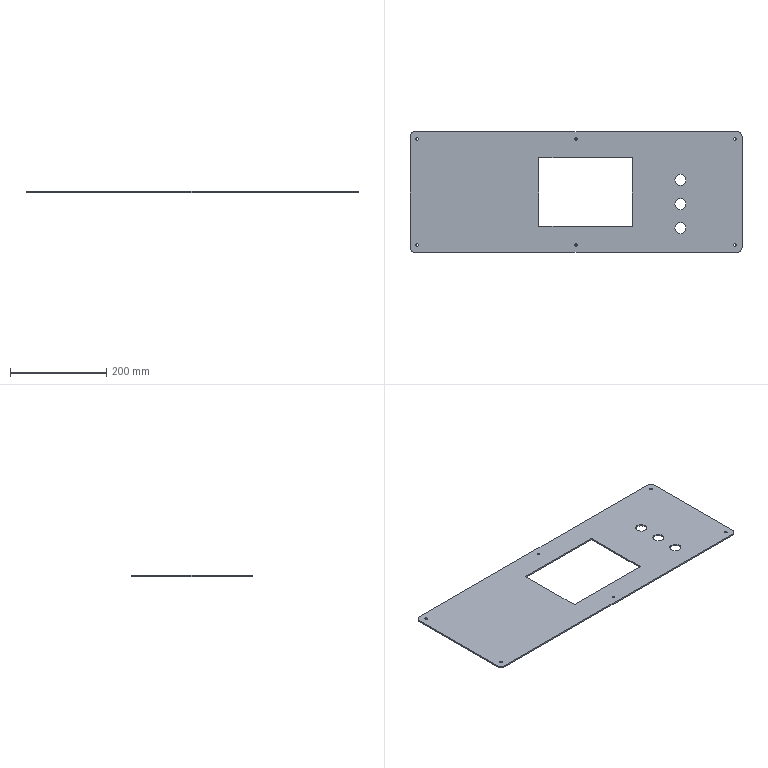Part | SolidWorks | features ICE 2, Extrusion 1, Fillet 1, HoleWzd 1 | 1 solid | 32 faces | box 690 x 250 x 3 mm | volume 429850 mm3 | cylinder 22 | plane 10 | commonest cylinder face diameters 5.5 x12 23 x6 20 x4
STEP:
#1=CARTESIAN_POINT('',(-332.75,110.,-1.5));
#2=VERTEX_POINT('',#1);
#3=CARTESIAN_POINT('',(-327.25,110.,-1.5));
#4=VERTEX_POINT('',#3);
#5=CARTESIAN_POINT('',(-330.,110.,-1.5));
#6=DIRECTION('',(0.,0.,1.));
#7=DIRECTION('',(1.,0.,0.));
#8=AXIS2_PLACEMENT_3D('',#5,#6,#7);
#9=CIRCLE('',#8,2.75);
#10=EDGE_CURVE('',#2,#4,#9,.T.);
#11=ORIENTED_EDGE('',*,*,#10,.F.);
#12=CARTESIAN_POINT('',(-332.75,110.,1.5));
#13=VERTEX_POINT('',#12);
#14=CARTESIAN_POINT('',(-332.75,110.,1.5));
#15=DIRECTION('',(0.,0.,1.));
#16=VECTOR('',#15,1000.);
#17=LINE('',#14,#16);
#18=EDGE_CURVE('',#2,#13,#17,.T.);
#19=ORIENTED_EDGE('',*,*,#18,.T.);
#20=CARTESIAN_POINT('',(-327.25,110.,1.5));
#21=VERTEX_POINT('',#20);
#22=CARTESIAN_POINT('',(-330.,110.,1.5));
#23=DIRECTION('',(0.,0.,1.));
#24=DIRECTION('',(1.,0.,0.));
#25=AXIS2_PLACEMENT_3D('',#22,#23,#24);
#26=CIRCLE('',#25,2.75);
#27=EDGE_CURVE('',#13,#21,#26,.T.);
#28=ORIENTED_EDGE('',*,*,#27,.T.);
#29=CARTESIAN_POINT('',(-327.25,110.,1.5));
#30=DIRECTION('',(0.,0.,1.));
#31=VECTOR('',#30,1000.);
#32=LINE('',#29,#31);
#33=EDGE_CURVE('',#4,#21,#32,.T.);
#34=ORIENTED_EDGE('',*,*,#33,.F.);
#35=EDGE_LOOP('',(#11,#19,#28,#34));
#36=FACE_OUTER_BOUND('',#35,.T.);
#37=CARTESIAN_POINT('',(-330.,110.,1.5));
#38=DIRECTION('',(0.,0.,1.));
#39=DIRECTION('',(1.,0.,0.));
#40=AXIS2_PLACEMENT_3D('',#37,#38,#39);
#41=CYLINDRICAL_SURFACE('',#40,2.75);
#42=ADVANCED_FACE('',(#36),#41,.F.);
#43=CARTESIAN_POINT('',(-2.75,110.,-1.5));
#44=VERTEX_POINT('',#43);
#45=CARTESIAN_POINT('',(2.75,110.,-1.5));
#46=VERTEX_POINT('',#45);
#47=CARTESIAN_POINT('',(0.,110.,-1.5));
#48=DIRECTION('',(0.,0.,1.));
#49=DIRECTION('',(1.,0.,0.));
#50=AXIS2_PLACEMENT_3D('',#47,#48,#49);
#51=CIRCLE('',#50,2.75);
#52=EDGE_CURVE('',#44,#46,#51,.T.);
#53=ORIENTED_EDGE('',*,*,#52,.F.);
#54=CARTESIAN_POINT('',(-2.75,110.,1.5));
#55=VERTEX_POINT('',#54);
#56=CARTESIAN_POINT('',(-2.75,110.,1.5));
#57=DIRECTION('',(0.,0.,1.));
#58=VECTOR('',#57,1000.);
#59=LINE('',#56,#58);
#60=EDGE_CURVE('',#44,#55,#59,.T.);
#61=ORIENTED_EDGE('',*,*,#60,.T.);
#62=CARTESIAN_POINT('',(2.75,110.,1.5));
#63=VERTEX_POINT('',#62);
#64=CARTESIAN_POINT('',(0.,110.,1.5));
#65=DIRECTION('',(0.,0.,1.));
#66=DIRECTION('',(1.,0.,0.));
#67=AXIS2_PLACEMENT_3D('',#64,#65,#66);
#68=CIRCLE('',#67,2.75);
#69=EDGE_CURVE('',#55,#63,#68,.T.);
#70=ORIENTED_EDGE('',*,*,#69,.T.);
#71=CARTESIAN_POINT('',(2.75,110.,1.5));
#72=DIRECTION('',(0.,0.,1.));
#73=VECTOR('',#72,1000.);
#74=LINE('',#71,#73);
#75=EDGE_CURVE('',#46,#63,#74,.T.);
#76=ORIENTED_EDGE('',*,*,#75,.F.);
#77=EDGE_LOOP('',(#53,#61,#70,#76));
#78=FACE_OUTER_BOUND('',#77,.T.);
#79=CARTESIAN_POINT('',(0.,110.,1.5));
#80=DIRECTION('',(0.,0.,1.));
#81=DIRECTION('',(1.,0.,0.));
#82=AXIS2_PLACEMENT_3D('',#79,#80,#81);
#83=CYLINDRICAL_SURFACE('',#82,2.75);
#84=ADVANCED_FACE('',(#78),#83,.F.);
#85=CARTESIAN_POINT('',(327.25,110.,-1.5));
#86=VERTEX_POINT('',#85);
#87=CARTESIAN_POINT('',(332.75,110.,-1.5));
#88=VERTEX_POINT('',#87);
#89=CARTESIAN_POINT('',(330.,110.,-1.5));
#90=DIRECTION('',(0.,0.,1.));
#91=DIRECTION('',(1.,0.,0.));
#92=AXIS2_PLACEMENT_3D('',#89,#90,#91);
#93=CIRCLE('',#92,2.75);
#94=EDGE_CURVE('',#86,#88,#93,.T.);
#95=ORIENTED_EDGE('',*,*,#94,.F.);
#96=CARTESIAN_POINT('',(327.25,110.,1.5));
#97=VERTEX_POINT('',#96);
#98=CARTESIAN_POINT('',(327.25,110.,1.5));
#99=DIRECTION('',(0.,0.,1.));
#100=VECTOR('',#99,1000.);
#101=LINE('',#98,#100);
#102=EDGE_CURVE('',#86,#97,#101,.T.);
#103=ORIENTED_EDGE('',*,*,#102,.T.);
#104=CARTESIAN_POINT('',(332.75,110.,1.5));
#105=VERTEX_POINT('',#104);
#106=CARTESIAN_POINT('',(330.,110.,1.5));
#107=DIRECTION('',(0.,0.,1.));
#108=DIRECTION('',(1.,0.,0.));
#109=AXIS2_PLACEMENT_3D('',#106,#107,#108);
#110=CIRCLE('',#109,2.75);
#111=EDGE_CURVE('',#97,#105,#110,.T.);
#112=ORIENTED_EDGE('',*,*,#111,.T.);
#113=CARTESIAN_POINT('',(332.75,110.,1.5));
#114=DIRECTION('',(0.,0.,1.));
#115=VECTOR('',#114,1000.);
#116=LINE('',#113,#115);
#117=EDGE_CURVE('',#88,#105,#116,.T.);
#118=ORIENTED_EDGE('',*,*,#117,.F.);
#119=EDGE_LOOP('',(#95,#103,#112,#118));
#120=FACE_OUTER_BOUND('',#119,.T.);
#121=CARTESIAN_POINT('',(330.,110.,1.5));
#122=DIRECTION('',(0.,0.,1.));
#123=DIRECTION('',(1.,0.,0.));
#124=AXIS2_PLACEMENT_3D('',#121,#122,#123);
#125=CYLINDRICAL_SURFACE('',#124,2.75);
#126=ADVANCED_FACE('',(#120),#125,.F.);
#127=CARTESIAN_POINT('',(327.25,-110.,-1.5));
#128=VERTEX_POINT('',#127);
#129=CARTESIAN_POINT('',(332.75,-110.,-1.5));
#130=VERTEX_POINT('',#129);
#131=CARTESIAN_POINT('',(330.,-110.,-1.5));
#132=DIRECTION('',(0.,0.,1.));
#133=DIRECTION('',(1.,0.,0.));
#134=AXIS2_PLACEMENT_3D('',#131,#132,#133);
#135=CIRCLE('',#134,2.75);
#136=EDGE_CURVE('',#128,#130,#135,.T.);
#137=ORIENTED_EDGE('',*,*,#136,.F.);
#138=CARTESIAN_POINT('',(327.25,-110.,1.5));
#139=VERTEX_POINT('',#138);
#140=CARTESIAN_POINT('',(327.25,-110.,1.5));
#141=DIRECTION('',(0.,0.,1.));
#142=VECTOR('',#141,1000.);
#143=LINE('',#140,#142);
#144=EDGE_CURVE('',#128,#139,#143,.T.);
#145=ORIENTED_EDGE('',*,*,#144,.T.);
#146=CARTESIAN_POINT('',(332.75,-110.,1.5));
#147=VERTEX_POINT('',#146);
#148=CARTESIAN_POINT('',(330.,-110.,1.5));
#149=DIRECTION('',(0.,0.,1.));
#150=DIRECTION('',(1.,0.,0.));
#151=AXIS2_PLACEMENT_3D('',#148,#149,#150);
#152=CIRCLE('',#151,2.75);
#153=EDGE_CURVE('',#139,#147,#152,.T.);
#154=ORIENTED_EDGE('',*,*,#153,.T.);
#155=CARTESIAN_POINT('',(332.75,-110.,1.5));
#156=DIRECTION('',(0.,0.,1.));
#157=VECTOR('',#156,1000.);
#158=LINE('',#155,#157);
#159=EDGE_CURVE('',#130,#147,#158,.T.);
#160=ORIENTED_EDGE('',*,*,#159,.F.);
#161=EDGE_LOOP('',(#137,#145,#154,#160));
#162=FACE_OUTER_BOUND('',#161,.T.);
#163=CARTESIAN_POINT('',(330.,-110.,1.5));
#164=DIRECTION('',(0.,0.,1.));
#165=DIRECTION('',(1.,0.,0.));
#166=AXIS2_PLACEMENT_3D('',#163,#164,#165);
#167=CYLINDRICAL_SURFACE('',#166,2.75);
#168=ADVANCED_FACE('',(#162),#167,.F.);
#169=CARTESIAN_POINT('',(-2.75,-110.,-1.5));
#170=VERTEX_POINT('',#169);
#171=CARTESIAN_POINT('',(2.75,-110.,-1.5));
#172=VERTEX_POINT('',#171);
#173=CARTESIAN_POINT('',(0.,-110.,-1.5));
#174=DIRECTION('',(0.,0.,1.));
#175=DIRECTION('',(1.,0.,0.));
#176=AXIS2_PLACEMENT_3D('',#173,#174,#175);
#177=CIRCLE('',#176,2.75);
#178=EDGE_CURVE('',#170,#172,#177,.T.);
#179=ORIENTED_EDGE('',*,*,#178,.F.);
#180=CARTESIAN_POINT('',(-2.75,-110.,1.5));
#181=VERTEX_POINT('',#180);
#182=CARTESIAN_POINT('',(-2.75,-110.,1.5));
#183=DIRECTION('',(0.,0.,1.));
#184=VECTOR('',#183,1000.);
#185=LINE('',#182,#184);
#186=EDGE_CURVE('',#170,#181,#185,.T.);
#187=ORIENTED_EDGE('',*,*,#186,.T.);
#188=CARTESIAN_POINT('',(2.75,-110.,1.5));
#189=VERTEX_POINT('',#188);
#190=CARTESIAN_POINT('',(0.,-110.,1.5));
#191=DIRECTION('',(0.,0.,1.));
#192=DIRECTION('',(1.,0.,0.));
#193=AXIS2_PLACEMENT_3D('',#190,#191,#192);
#194=CIRCLE('',#193,2.75);
#195=EDGE_CURVE('',#181,#189,#194,.T.);
#196=ORIENTED_EDGE('',*,*,#195,.T.);
#197=CARTESIAN_POINT('',(2.75,-110.,1.5));
#198=DIRECTION('',(0.,0.,1.));
#199=VECTOR('',#198,1000.);
#200=LINE('',#197,#199);
#201=EDGE_CURVE('',#172,#189,#200,.T.);
#202=ORIENTED_EDGE('',*,*,#201,.F.);
#203=EDGE_LOOP('',(#179,#187,#196,#202));
#204=FACE_OUTER_BOUND('',#203,.T.);
#205=CARTESIAN_POINT('',(0.,-110.,1.5));
#206=DIRECTION('',(0.,0.,1.));
#207=DIRECTION('',(1.,0.,0.));
#208=AXIS2_PLACEMENT_3D('',#205,#206,#207);
#209=CYLINDRICAL_SURFACE('',#208,2.75);
#210=ADVANCED_FACE('',(#204),#209,.F.);
#211=CARTESIAN_POINT('',(-332.75,-110.,-1.5));
#212=VERTEX_POINT('',#211);
#213=CARTESIAN_POINT('',(-327.25,-110.,-1.5));
#214=VERTEX_POINT('',#213);
#215=CARTESIAN_POINT('',(-330.,-110.,-1.5));
#216=DIRECTION('',(0.,0.,1.));
#217=DIRECTION('',(1.,0.,0.));
#218=AXIS2_PLACEMENT_3D('',#215,#216,#217);
#219=CIRCLE('',#218,2.75);
#220=EDGE_CURVE('',#212,#214,#219,.T.);
#221=ORIENTED_EDGE('',*,*,#220,.F.);
#222=CARTESIAN_POINT('',(-332.75,-110.,1.5));
#223=VERTEX_POINT('',#222);
#224=CARTESIAN_POINT('',(-332.75,-110.,1.5));
#225=DIRECTION('',(0.,0.,1.));
#226=VECTOR('',#225,1000.);
#227=LINE('',#224,#226);
#228=EDGE_CURVE('',#212,#223,#227,.T.);
#229=ORIENTED_EDGE('',*,*,#228,.T.);
#230=CARTESIAN_POINT('',(-327.25,-110.,1.5));
#231=VERTEX_POINT('',#230);
#232=CARTESIAN_POINT('',(-330.,-110.,1.5));
#233=DIRECTION('',(0.,0.,1.));
#234=DIRECTION('',(1.,0.,0.));
#235=AXIS2_PLACEMENT_3D('',#232,#233,#234);
#236=CIRCLE('',#235,2.75);
#237=EDGE_CURVE('',#223,#231,#236,.T.);
#238=ORIENTED_EDGE('',*,*,#237,.T.);
#239=CARTESIAN_POINT('',(-327.25,-110.,1.5));
#240=DIRECTION('',(0.,0.,1.));
#241=VECTOR('',#240,1000.);
#242=LINE('',#239,#241);
#243=EDGE_CURVE('',#214,#231,#242,.T.);
#244=ORIENTED_EDGE('',*,*,#243,.F.);
#245=EDGE_LOOP('',(#221,#229,#238,#244));
#246=FACE_OUTER_BOUND('',#245,.T.);
#247=CARTESIAN_POINT('',(-330.,-110.,1.5));
#248=DIRECTION('',(0.,0.,1.));
#249=DIRECTION('',(1.,0.,0.));
#250=AXIS2_PLACEMENT_3D('',#247,#248,#249);
#251=CYLINDRICAL_SURFACE('',#250,2.75);
#252=ADVANCED_FACE('',(#246),#251,.F.);
#253=CARTESIAN_POINT('',(205.5,25.,-1.5));
#254=VERTEX_POINT('',#253);
#255=CARTESIAN_POINT('',(228.5,25.,-1.5));
#256=VERTEX_POINT('',#255);
#257=CARTESIAN_POINT('',(217.,25.,-1.5));
#258=DIRECTION('',(0.,0.,1.));
#259=DIRECTION('',(1.,0.,0.));
#260=AXIS2_PLACEMENT_3D('',#257,#258,#259);
#261=CIRCLE('',#260,11.5);
#262=EDGE_CURVE('',#254,#256,#261,.T.);
#263=ORIENTED_EDGE('',*,*,#262,.F.);
#264=CARTESIAN_POINT('',(205.5,25.,1.5));
#265=VERTEX_POINT('',#264);
#266=CARTESIAN_POINT('',(205.5,25.,-4.5));
#267=DIRECTION('',(0.,0.,1.));
#268=VECTOR('',#267,1000.);
#269=LINE('',#266,#268);
#270=EDGE_CURVE('',#254,#265,#269,.T.);
#271=ORIENTED_EDGE('',*,*,#270,.T.);
#272=CARTESIAN_POINT('',(228.5,25.,1.5));
#273=VERTEX_POINT('',#272);
#274=CARTESIAN_POINT('',(217.,25.,1.5));
#275=DIRECTION('',(0.,0.,1.));
#276=DIRECTION('',(1.,0.,0.));
#277=AXIS2_PLACEMENT_3D('',#274,#275,#276);
#278=CIRCLE('',#277,11.5);
#279=EDGE_CURVE('',#265,#273,#278,.T.);
#280=ORIENTED_EDGE('',*,*,#279,.T.);
#281=CARTESIAN_POINT('',(228.5,25.,-4.5));
#282=DIRECTION('',(0.,0.,1.));
#283=VECTOR('',#282,1000.);
#284=LINE('',#281,#283);
#285=EDGE_CURVE('',#256,#273,#284,.T.);
#286=ORIENTED_EDGE('',*,*,#285,.F.);
#287=EDGE_LOOP('',(#263,#271,#280,#286));
#288=FACE_OUTER_BOUND('',#287,.T.);
#289=CARTESIAN_POINT('',(217.,25.,-4.5));
#290=DIRECTION('',(0.,0.,1.));
#291=DIRECTION('',(1.,0.,0.));
#292=AXIS2_PLACEMENT_3D('',#289,#290,#291);
#293=CYLINDRICAL_SURFACE('',#292,11.5);
#294=ADVANCED_FACE('',(#288),#293,.F.);
#295=CARTESIAN_POINT('',(205.5,-75.,-1.5));
#296=VERTEX_POINT('',#295);
#297=CARTESIAN_POINT('',(228.5,-75.,-1.5));
#298=VERTEX_POINT('',#297);
#299=CARTESIAN_POINT('',(217.,-75.,-1.5));
#300=DIRECTION('',(0.,0.,1.));
#301=DIRECTION('',(1.,0.,0.));
#302=AXIS2_PLACEMENT_3D('',#299,#300,#301);
#303=CIRCLE('',#302,11.5);
#304=EDGE_CURVE('',#296,#298,#303,.T.);
#305=ORIENTED_EDGE('',*,*,#304,.F.);
#306=CARTESIAN_POINT('',(205.5,-75.,1.5));
#307=VERTEX_POINT('',#306);
#308=CARTESIAN_POINT('',(205.5,-75.,-4.5));
#309=DIRECTION('',(0.,0.,1.));
#310=VECTOR('',#309,1000.);
#311=LINE('',#308,#310);
#312=EDGE_CURVE('',#296,#307,#311,.T.);
#313=ORIENTED_EDGE('',*,*,#312,.T.);
#314=CARTESIAN_POINT('',(228.5,-75.,1.5));
#315=VERTEX_POINT('',#314);
#316=CARTESIAN_POINT('',(217.,-75.,1.5));
#317=DIRECTION('',(0.,0.,1.));
#318=DIRECTION('',(1.,0.,0.));
#319=AXIS2_PLACEMENT_3D('',#316,#317,#318);
#320=CIRCLE('',#319,11.5);
#321=EDGE_CURVE('',#307,#315,#320,.T.);
#322=ORIENTED_EDGE('',*,*,#321,.T.);
#323=CARTESIAN_POINT('',(228.5,-75.,-4.5));
#324=DIRECTION('',(0.,0.,1.));
#325=VECTOR('',#324,1000.);
#326=LINE('',#323,#325);
#327=EDGE_CURVE('',#298,#315,#326,.T.);
#328=ORIENTED_EDGE('',*,*,#327,.F.);
#329=EDGE_LOOP('',(#305,#313,#322,#328));
#330=FACE_OUTER_BOUND('',#329,.T.);
#331=CARTESIAN_POINT('',(217.,-75.,-4.5));
#332=DIRECTION('',(0.,0.,1.));
#333=DIRECTION('',(1.,0.,0.));
#334=AXIS2_PLACEMENT_3D('',#331,#332,#333);
#335=CYLINDRICAL_SURFACE('',#334,11.5);
#336=ADVANCED_FACE('',(#330),#335,.F.);
#337=CARTESIAN_POINT('',(205.5,-25.,-1.5));
#338=VERTEX_POINT('',#337);
#339=CARTESIAN_POINT('',(228.5,-25.,-1.5));
#340=VERTEX_POINT('',#339);
#341=CARTESIAN_POINT('',(217.,-25.,-1.5));
#342=DIRECTION('',(0.,0.,1.));
#343=DIRECTION('',(1.,0.,0.));
#344=AXIS2_PLACEMENT_3D('',#341,#342,#343);
#345=CIRCLE('',#344,11.5);
#346=EDGE_CURVE('',#338,#340,#345,.T.);
#347=ORIENTED_EDGE('',*,*,#346,.F.);
#348=CARTESIAN_POINT('',(205.5,-25.,1.5));
#349=VERTEX_POINT('',#348);
#350=CARTESIAN_POINT('',(205.5,-25.,-4.5));
#351=DIRECTION('',(0.,0.,1.));
#352=VECTOR('',#351,1000.);
#353=LINE('',#350,#352);
#354=EDGE_CURVE('',#338,#349,#353,.T.);
#355=ORIENTED_EDGE('',*,*,#354,.T.);
#356=CARTESIAN_POINT('',(228.5,-25.,1.5));
#357=VERTEX_POINT('',#356);
#358=CARTESIAN_POINT('',(217.,-25.,1.5));
#359=DIRECTION('',(0.,0.,1.));
#360=DIRECTION('',(1.,0.,0.));
#361=AXIS2_PLACEMENT_3D('',#358,#359,#360);
#362=CIRCLE('',#361,11.5);
#363=EDGE_CURVE('',#349,#357,#362,.T.);
#364=ORIENTED_EDGE('',*,*,#363,.T.);
#365=CARTESIAN_POINT('',(228.5,-25.,-4.5));
#366=DIRECTION('',(0.,0.,1.));
#367=VECTOR('',#366,1000.);
#368=LINE('',#365,#367);
#369=EDGE_CURVE('',#340,#357,#368,.T.);
#370=ORIENTED_EDGE('',*,*,#369,.F.);
#371=EDGE_LOOP('',(#347,#355,#364,#370));
#372=FACE_OUTER_BOUND('',#371,.T.);
#373=CARTESIAN_POINT('',(217.,-25.,-4.5));
#374=DIRECTION('',(0.,0.,1.));
#375=DIRECTION('',(1.,0.,0.));
#376=AXIS2_PLACEMENT_3D('',#373,#374,#375);
#377=CYLINDRICAL_SURFACE('',#376,11.5);
#378=ADVANCED_FACE('',(#372),#377,.F.);
#379=CARTESIAN_POINT('',(345.,-115.,1.5));
#380=VERTEX_POINT('',#379);
#381=CARTESIAN_POINT('',(345.,115.,1.5));
#382=VERTEX_POINT('',#381);
#383=CARTESIAN_POINT('',(345.,125.,1.5));
#384=DIRECTION('',(0.,1.,0.));
#385=VECTOR('',#384,1000.);
#386=LINE('',#383,#385);
#387=EDGE_CURVE('',#380,#382,#386,.T.);
#388=ORIENTED_EDGE('',*,*,#387,.F.);
#389=CARTESIAN_POINT('',(345.,-115.,-1.5));
#390=VERTEX_POINT('',#389);
#391=CARTESIAN_POINT('',(345.,-115.,1.5));
#392=DIRECTION('',(0.,0.,-1.));
#393=VECTOR('',#392,1000.);
#394=LINE('',#391,#393);
#395=EDGE_CURVE('',#380,#390,#394,.T.);
#396=ORIENTED_EDGE('',*,*,#395,.T.);
#397=CARTESIAN_POINT('',(345.,115.,-1.5));
#398=VERTEX_POINT('',#397);
#399=CARTESIAN_POINT('',(345.,125.,-1.5));
#400=DIRECTION('',(0.,1.,0.));
#401=VECTOR('',#400,1000.);
#402=LINE('',#399,#401);
#403=EDGE_CURVE('',#390,#398,#402,.T.);
#404=ORIENTED_EDGE('',*,*,#403,.T.);
#405=CARTESIAN_POINT('',(345.,115.,1.5));
#406=DIRECTION('',(0.,0.,1.));
#407=VECTOR('',#406,1000.);
#408=LINE('',#405,#407);
#409=EDGE_CURVE('',#398,#382,#408,.T.);
#410=ORIENTED_EDGE('',*,*,#409,.T.);
#411=EDGE_LOOP('',(#388,#396,#404,#410));
#412=FACE_OUTER_BOUND('',#411,.T.);
#413=CARTESIAN_POINT('',(345.,125.,1.5));
#414=DIRECTION('',(-1.,0.,0.));
#415=DIRECTION('',(0.,0.,1.));
#416=AXIS2_PLACEMENT_3D('',#413,#414,#415);
#417=PLANE('',#416);
#418=ADVANCED_FACE('',(#412),#417,.F.);
#419=CARTESIAN_POINT('',(335.,125.,1.5));
#420=VERTEX_POINT('',#419);
#421=CARTESIAN_POINT('',(-335.,125.,1.5));
#422=VERTEX_POINT('',#421);
#423=CARTESIAN_POINT('',(-345.,125.,1.5));
#424=DIRECTION('',(-1.,0.,0.));
#425=VECTOR('',#424,1000.);
#426=LINE('',#423,#425);
#427=EDGE_CURVE('',#420,#422,#426,.T.);
#428=ORIENTED_EDGE('',*,*,#427,.F.);
#429=CARTESIAN_POINT('',(335.,125.,-1.5));
#430=VERTEX_POINT('',#429);
#431=CARTESIAN_POINT('',(335.,125.,1.5));
#432=DIRECTION('',(0.,0.,-1.));
#433=VECTOR('',#432,1000.);
#434=LINE('',#431,#433);
#435=EDGE_CURVE('',#420,#430,#434,.T.);
#436=ORIENTED_EDGE('',*,*,#435,.T.);
#437=CARTESIAN_POINT('',(-335.,125.,-1.5));
#438=VERTEX_POINT('',#437);
#439=CARTESIAN_POINT('',(-345.,125.,-1.5));
#440=DIRECTION('',(-1.,0.,0.));
#441=VECTOR('',#440,1000.);
#442=LINE('',#439,#441);
#443=EDGE_CURVE('',#430,#438,#442,.T.);
#444=ORIENTED_EDGE('',*,*,#443,.T.);
#445=CARTESIAN_POINT('',(-335.,125.,1.5));
#446=DIRECTION('',(0.,0.,1.));
#447=VECTOR('',#446,1000.);
#448=LINE('',#445,#447);
#449=EDGE_CURVE('',#438,#422,#448,.T.);
#450=ORIENTED_EDGE('',*,*,#449,.T.);
#451=EDGE_LOOP('',(#428,#436,#444,#450));
#452=FACE_OUTER_BOUND('',#451,.T.);
#453=CARTESIAN_POINT('',(-345.,125.,1.5));
#454=DIRECTION('',(0.,-1.,0.));
#455=DIRECTION('',(0.,0.,-1.));
#456=AXIS2_PLACEMENT_3D('',#453,#454,#455);
#457=PLANE('',#456);
#458=ADVANCED_FACE('',(#452),#457,.F.);
#459=CARTESIAN_POINT('',(-345.,115.,-1.5));
#460=VERTEX_POINT('',#459);
#461=CARTESIAN_POINT('',(-345.,-115.,-1.5));
#462=VERTEX_POINT('',#461);
#463=CARTESIAN_POINT('',(-345.,125.,-1.5));
#464=DIRECTION('',(0.,-1.,0.));
#465=VECTOR('',#464,1000.);
#466=LINE('',#463,#465);
#467=EDGE_CURVE('',#460,#462,#466,.T.);
#468=ORIENTED_EDGE('',*,*,#467,.T.);
#469=CARTESIAN_POINT('',(-345.,-115.,1.5));
#470=VERTEX_POINT('',#469);
#471=CARTESIAN_POINT('',(-345.,-115.,1.5));
#472=DIRECTION('',(0.,0.,1.));
#473=VECTOR('',#472,1000.);
#474=LINE('',#471,#473);
#475=EDGE_CURVE('',#462,#470,#474,.T.);
#476=ORIENTED_EDGE('',*,*,#475,.T.);
#477=CARTESIAN_POINT('',(-345.,115.,1.5));
#478=VERTEX_POINT('',#477);
#479=CARTESIAN_POINT('',(-345.,125.,1.5));
#480=DIRECTION('',(0.,-1.,0.));
#481=VECTOR('',#480,1000.);
#482=LINE('',#479,#481);
#483=EDGE_CURVE('',#478,#470,#482,.T.);
#484=ORIENTED_EDGE('',*,*,#483,.F.);
#485=CARTESIAN_POINT('',(-345.,115.,1.5));
#486=DIRECTION('',(0.,0.,-1.));
#487=VECTOR('',#486,1000.);
#488=LINE('',#485,#487);
#489=EDGE_CURVE('',#478,#460,#488,.T.);
#490=ORIENTED_EDGE('',*,*,#489,.T.);
#491=EDGE_LOOP('',(#468,#476,#484,#490));
#492=FACE_OUTER_BOUND('',#491,.T.);
#493=CARTESIAN_POINT('',(-345.,125.,1.5));
#494=DIRECTION('',(1.,0.,0.));
#495=DIRECTION('',(0.,1.,0.));
#496=AXIS2_PLACEMENT_3D('',#493,#494,#495);
#497=PLANE('',#496);
#498=ADVANCED_FACE('',(#492),#497,.F.);
#499=CARTESIAN_POINT('',(-335.,-125.,-1.5));
#500=VERTEX_POINT('',#499);
#501=CARTESIAN_POINT('',(335.,-125.,-1.5));
#502=VERTEX_POINT('',#501);
#503=CARTESIAN_POINT('',(-345.,-125.,-1.5));
#504=DIRECTION('',(1.,0.,0.));
#505=VECTOR('',#504,1000.);
#506=LINE('',#503,#505);
#507=EDGE_CURVE('',#500,#502,#506,.T.);
#508=ORIENTED_EDGE('',*,*,#507,.T.);
#509=CARTESIAN_POINT('',(335.,-125.,1.5));
#510=VERTEX_POINT('',#509);
#511=CARTESIAN_POINT('',(335.,-125.,1.5));
#512=DIRECTION('',(0.,0.,1.));
#513=VECTOR('',#512,1000.);
#514=LINE('',#511,#513);
#515=EDGE_CURVE('',#502,#510,#514,.T.);
#516=ORIENTED_EDGE('',*,*,#515,.T.);
#517=CARTESIAN_POINT('',(-335.,-125.,1.5));
#518=VERTEX_POINT('',#517);
#519=CARTESIAN_POINT('',(-345.,-125.,1.5));
#520=DIRECTION('',(1.,0.,0.));
#521=VECTOR('',#520,1000.);
#522=LINE('',#519,#521);
#523=EDGE_CURVE('',#518,#510,#522,.T.);
#524=ORIENTED_EDGE('',*,*,#523,.F.);
#525=CARTESIAN_POINT('',(-335.,-125.,1.5));
#526=DIRECTION('',(0.,0.,-1.));
#527=VECTOR('',#526,1000.);
#528=LINE('',#525,#527);
#529=EDGE_CURVE('',#518,#500,#528,.T.);
#530=ORIENTED_EDGE('',*,*,#529,.T.);
#531=EDGE_LOOP('',(#508,#516,#524,#530));
#532=FACE_OUTER_BOUND('',#531,.T.);
#533=CARTESIAN_POINT('',(-345.,-125.,1.5));
#534=DIRECTION('',(0.,1.,0.));
#535=DIRECTION('',(0.,0.,1.));
#536=AXIS2_PLACEMENT_3D('',#533,#534,#535);
#537=PLANE('',#536);
#538=ADVANCED_FACE('',(#532),#537,.F.);
#539=CARTESIAN_POINT('',(-330.,110.,1.5));
#540=DIRECTION('',(0.,0.,1.));
#541=DIRECTION('',(1.,0.,0.));
#542=AXIS2_PLACEMENT_3D('',#539,#540,#541);
#543=CIRCLE('',#542,2.75);
#544=EDGE_CURVE('',#21,#13,#543,.T.);
#545=ORIENTED_EDGE('',*,*,#544,.F.);
#546=ORIENTED_EDGE('',*,*,#27,.F.);
#547=EDGE_LOOP('',(#545,#546));
#548=FACE_BOUND('',#547,.T.);
#549=CARTESIAN_POINT('',(0.,110.,1.5));
#550=DIRECTION('',(0.,0.,1.));
#551=DIRECTION('',(1.,0.,0.));
#552=AXIS2_PLACEMENT_3D('',#549,#550,#551);
#553=CIRCLE('',#552,2.75);
#554=EDGE_CURVE('',#63,#55,#553,.T.);
#555=ORIENTED_EDGE('',*,*,#554,.F.);
#556=ORIENTED_EDGE('',*,*,#69,.F.);
#557=EDGE_LOOP('',(#555,#556));
#558=FACE_BOUND('',#557,.T.);
#559=CARTESIAN_POINT('',(330.,110.,1.5));
#560=DIRECTION('',(0.,0.,1.));
#561=DIRECTION('',(1.,0.,0.));
#562=AXIS2_PLACEMENT_3D('',#559,#560,#561);
#563=CIRCLE('',#562,2.75);
#564=EDGE_CURVE('',#105,#97,#563,.T.);
#565=ORIENTED_EDGE('',*,*,#564,.F.);
#566=ORIENTED_EDGE('',*,*,#111,.F.);
#567=EDGE_LOOP('',(#565,#566));
#568=FACE_BOUND('',#567,.T.);
#569=CARTESIAN_POINT('',(330.,-110.,1.5));
#570=DIRECTION('',(0.,0.,1.));
#571=DIRECTION('',(1.,0.,0.));
#572=AXIS2_PLACEMENT_3D('',#569,#570,#571);
#573=CIRCLE('',#572,2.75);
#574=EDGE_CURVE('',#147,#139,#573,.T.);
#575=ORIENTED_EDGE('',*,*,#574,.F.);
#576=ORIENTED_EDGE('',*,*,#153,.F.);
#577=EDGE_LOOP('',(#575,#576));
#578=FACE_BOUND('',#577,.T.);
#579=CARTESIAN_POINT('',(0.,-110.,1.5));
#580=DIRECTION('',(0.,0.,1.));
#581=DIRECTION('',(1.,0.,0.));
#582=AXIS2_PLACEMENT_3D('',#579,#580,#581);
#583=CIRCLE('',#582,2.75);
#584=EDGE_CURVE('',#189,#181,#583,.T.);
#585=ORIENTED_EDGE('',*,*,#584,.F.);
#586=ORIENTED_EDGE('',*,*,#195,.F.);
#587=EDGE_LOOP('',(#585,#586));
#588=FACE_BOUND('',#587,.T.);
#589=CARTESIAN_POINT('',(-330.,-110.,1.5));
#590=DIRECTION('',(0.,0.,1.));
#591=DIRECTION('',(1.,0.,0.));
#592=AXIS2_PLACEMENT_3D('',#589,#590,#591);
#593=CIRCLE('',#592,2.75);
#594=EDGE_CURVE('',#231,#223,#593,.T.);
#595=ORIENTED_EDGE('',*,*,#594,.F.);
#596=ORIENTED_EDGE('',*,*,#237,.F.);
#597=EDGE_LOOP('',(#595,#596));
#598=FACE_BOUND('',#597,.T.);
#599=CARTESIAN_POINT('',(217.,25.,1.5));
#600=DIRECTION('',(0.,0.,1.));
#601=DIRECTION('',(1.,0.,0.));
#602=AXIS2_PLACEMENT_3D('',#599,#600,#601);
#603=CIRCLE('',#602,11.5);
#604=EDGE_CURVE('',#273,#265,#603,.T.);
#605=ORIENTED_EDGE('',*,*,#604,.F.);
#606=ORIENTED_EDGE('',*,*,#279,.F.);
#607=EDGE_LOOP('',(#605,#606));
#608=FACE_BOUND('',#607,.T.);
#609=CARTESIAN_POINT('',(217.,-75.,1.5));
#610=DIRECTION('',(0.,0.,1.));
#611=DIRECTION('',(1.,0.,0.));
#612=AXIS2_PLACEMENT_3D('',#609,#610,#611);
#613=CIRCLE('',#612,11.5);
#614=EDGE_CURVE('',#315,#307,#613,.T.);
#615=ORIENTED_EDGE('',*,*,#614,.F.);
#616=ORIENTED_EDGE('',*,*,#321,.F.);
#617=EDGE_LOOP('',(#615,#616));
#618=FACE_BOUND('',#617,.T.);
#619=CARTESIAN_POINT('',(217.,-25.,1.5));
#620=DIRECTION('',(0.,0.,1.));
#621=DIRECTION('',(1.,0.,0.));
#622=AXIS2_PLACEMENT_3D('',#619,#620,#621);
#623=CIRCLE('',#622,11.5);
#624=EDGE_CURVE('',#357,#349,#623,.T.);
#625=ORIENTED_EDGE('',*,*,#624,.F.);
#626=ORIENTED_EDGE('',*,*,#363,.F.);
#627=EDGE_LOOP('',(#625,#626));
#628=FACE_BOUND('',#627,.T.);
#629=CARTESIAN_POINT('',(117.,-71.5,1.5));
#630=VERTEX_POINT('',#629);
#631=CARTESIAN_POINT('',(117.,71.5,1.5));
#632=VERTEX_POINT('',#631);
#633=CARTESIAN_POINT('',(117.,71.5,1.5));
#634=DIRECTION('',(0.,1.,0.));
#635=VECTOR('',#634,1000.);
#636=LINE('',#633,#635);
#637=EDGE_CURVE('',#630,#632,#636,.T.);
#638=ORIENTED_EDGE('',*,*,#637,.F.);
#639=CARTESIAN_POINT('',(-77.,-71.5,1.5));
#640=VERTEX_POINT('',#639);
#641=CARTESIAN_POINT('',(-77.,-71.5,1.5));
#642=DIRECTION('',(1.,0.,0.));
#643=VECTOR('',#642,1000.);
#644=LINE('',#641,#643);
#645=EDGE_CURVE('',#640,#630,#644,.T.);
#646=ORIENTED_EDGE('',*,*,#645,.F.);
#647=CARTESIAN_POINT('',(-77.,71.5,1.5));
#648=VERTEX_POINT('',#647);
#649=CARTESIAN_POINT('',(-77.,71.5,1.5));
#650=DIRECTION('',(0.,-1.,0.));
#651=VECTOR('',#650,1000.);
#652=LINE('',#649,#651);
#653=EDGE_CURVE('',#648,#640,#652,.T.);
#654=ORIENTED_EDGE('',*,*,#653,.F.);
#655=CARTESIAN_POINT('',(-77.,71.5,1.5));
#656=DIRECTION('',(-1.,0.,0.));
#657=VECTOR('',#656,1000.);
#658=LINE('',#655,#657);
#659=EDGE_CURVE('',#632,#648,#658,.T.);
#660=ORIENTED_EDGE('',*,*,#659,.F.);
#661=EDGE_LOOP('',(#638,#646,#654,#660));
#662=FACE_BOUND('',#661,.T.);
#663=ORIENTED_EDGE('',*,*,#523,.T.);
#664=CARTESIAN_POINT('',(335.,-115.,1.5));
#665=DIRECTION('',(0.,0.,1.));
#666=DIRECTION('',(1.,0.,0.));
#667=AXIS2_PLACEMENT_3D('',#664,#665,#666);
#668=CIRCLE('',#667,10.);
#669=EDGE_CURVE('',#510,#380,#668,.T.);
#670=ORIENTED_EDGE('',*,*,#669,.T.);
#671=ORIENTED_EDGE('',*,*,#387,.T.);
#672=CARTESIAN_POINT('',(335.,115.,1.5));
#673=DIRECTION('',(0.,0.,1.));
#674=DIRECTION('',(1.,0.,0.));
#675=AXIS2_PLACEMENT_3D('',#672,#673,#674);
#676=CIRCLE('',#675,10.);
#677=EDGE_CURVE('',#382,#420,#676,.T.);
#678=ORIENTED_EDGE('',*,*,#677,.T.);
#679=ORIENTED_EDGE('',*,*,#427,.T.);
#680=CARTESIAN_POINT('',(-335.,115.,1.5));
#681=DIRECTION('',(0.,0.,1.));
#682=DIRECTION('',(1.,0.,0.));
#683=AXIS2_PLACEMENT_3D('',#680,#681,#682);
#684=CIRCLE('',#683,10.);
#685=EDGE_CURVE('',#422,#478,#684,.T.);
#686=ORIENTED_EDGE('',*,*,#685,.T.);
#687=ORIENTED_EDGE('',*,*,#483,.T.);
#688=CARTESIAN_POINT('',(-335.,-115.,1.5));
#689=DIRECTION('',(0.,0.,1.));
#690=DIRECTION('',(1.,0.,0.));
#691=AXIS2_PLACEMENT_3D('',#688,#689,#690);
#692=CIRCLE('',#691,10.);
#693=EDGE_CURVE('',#470,#518,#692,.T.);
#694=ORIENTED_EDGE('',*,*,#693,.T.);
#695=EDGE_LOOP('',(#663,#670,#671,#678,#679,#686,#687,#694));
#696=FACE_OUTER_BOUND('',#695,.T.);
#697=CARTESIAN_POINT('',(345.,-125.,1.5));
#698=DIRECTION('',(0.,0.,1.));
#699=DIRECTION('',(1.,0.,0.));
#700=AXIS2_PLACEMENT_3D('',#697,#698,#699);
#701=PLANE('',#700);
#702=ADVANCED_FACE('',(#548,#558,#568,#578,#588,#598,#608,#618,#628,#662,#696),#701,.T.);
#703=CARTESIAN_POINT('',(-330.,110.,-1.5));
#704=DIRECTION('',(0.,0.,1.));
#705=DIRECTION('',(1.,0.,0.));
#706=AXIS2_PLACEMENT_3D('',#703,#704,#705);
#707=CIRCLE('',#706,2.75);
#708=EDGE_CURVE('',#4,#2,#707,.T.);
#709=ORIENTED_EDGE('',*,*,#708,.T.);
#710=ORIENTED_EDGE('',*,*,#10,.T.);
#711=EDGE_LOOP('',(#709,#710));
#712=FACE_BOUND('',#711,.T.);
#713=CARTESIAN_POINT('',(0.,110.,-1.5));
#714=DIRECTION('',(0.,0.,1.));
#715=DIRECTION('',(1.,0.,0.));
#716=AXIS2_PLACEMENT_3D('',#713,#714,#715);
#717=CIRCLE('',#716,2.75);
#718=EDGE_CURVE('',#46,#44,#717,.T.);
#719=ORIENTED_EDGE('',*,*,#718,.T.);
#720=ORIENTED_EDGE('',*,*,#52,.T.);
#721=EDGE_LOOP('',(#719,#720));
#722=FACE_BOUND('',#721,.T.);
#723=CARTESIAN_POINT('',(330.,110.,-1.5));
#724=DIRECTION('',(0.,0.,1.));
#725=DIRECTION('',(1.,0.,0.));
#726=AXIS2_PLACEMENT_3D('',#723,#724,#725);
#727=CIRCLE('',#726,2.75);
#728=EDGE_CURVE('',#88,#86,#727,.T.);
#729=ORIENTED_EDGE('',*,*,#728,.T.);
#730=ORIENTED_EDGE('',*,*,#94,.T.);
#731=EDGE_LOOP('',(#729,#730));
#732=FACE_BOUND('',#731,.T.);
#733=CARTESIAN_POINT('',(330.,-110.,-1.5));
#734=DIRECTION('',(0.,0.,1.));
#735=DIRECTION('',(1.,0.,0.));
#736=AXIS2_PLACEMENT_3D('',#733,#734,#735);
#737=CIRCLE('',#736,2.75);
#738=EDGE_CURVE('',#130,#128,#737,.T.);
#739=ORIENTED_EDGE('',*,*,#738,.T.);
#740=ORIENTED_EDGE('',*,*,#136,.T.);
#741=EDGE_LOOP('',(#739,#740));
#742=FACE_BOUND('',#741,.T.);
#743=CARTESIAN_POINT('',(0.,-110.,-1.5));
#744=DIRECTION('',(0.,0.,1.));
#745=DIRECTION('',(1.,0.,0.));
#746=AXIS2_PLACEMENT_3D('',#743,#744,#745);
#747=CIRCLE('',#746,2.75);
#748=EDGE_CURVE('',#172,#170,#747,.T.);
#749=ORIENTED_EDGE('',*,*,#748,.T.);
#750=ORIENTED_EDGE('',*,*,#178,.T.);
#751=EDGE_LOOP('',(#749,#750));
#752=FACE_BOUND('',#751,.T.);
#753=CARTESIAN_POINT('',(-330.,-110.,-1.5));
#754=DIRECTION('',(0.,0.,1.));
#755=DIRECTION('',(1.,0.,0.));
#756=AXIS2_PLACEMENT_3D('',#753,#754,#755);
#757=CIRCLE('',#756,2.75);
#758=EDGE_CURVE('',#214,#212,#757,.T.);
#759=ORIENTED_EDGE('',*,*,#758,.T.);
#760=ORIENTED_EDGE('',*,*,#220,.T.);
#761=EDGE_LOOP('',(#759,#760));
#762=FACE_BOUND('',#761,.T.);
#763=CARTESIAN_POINT('',(217.,25.,-1.5));
#764=DIRECTION('',(0.,0.,1.));
#765=DIRECTION('',(1.,0.,0.));
#766=AXIS2_PLACEMENT_3D('',#763,#764,#765);
#767=CIRCLE('',#766,11.5);
#768=EDGE_CURVE('',#256,#254,#767,.T.);
#769=ORIENTED_EDGE('',*,*,#768,.T.);
#770=ORIENTED_EDGE('',*,*,#262,.T.);
#771=EDGE_LOOP('',(#769,#770));
#772=FACE_BOUND('',#771,.T.);
#773=CARTESIAN_POINT('',(217.,-75.,-1.5));
#774=DIRECTION('',(0.,0.,1.));
#775=DIRECTION('',(1.,0.,0.));
#776=AXIS2_PLACEMENT_3D('',#773,#774,#775);
#777=CIRCLE('',#776,11.5);
#778=EDGE_CURVE('',#298,#296,#777,.T.);
#779=ORIENTED_EDGE('',*,*,#778,.T.);
#780=ORIENTED_EDGE('',*,*,#304,.T.);
#781=EDGE_LOOP('',(#779,#780));
#782=FACE_BOUND('',#781,.T.);
#783=CARTESIAN_POINT('',(217.,-25.,-1.5));
#784=DIRECTION('',(0.,0.,1.));
#785=DIRECTION('',(1.,0.,0.));
#786=AXIS2_PLACEMENT_3D('',#783,#784,#785);
#787=CIRCLE('',#786,11.5);
#788=EDGE_CURVE('',#340,#338,#787,.T.);
#789=ORIENTED_EDGE('',*,*,#788,.T.);
#790=ORIENTED_EDGE('',*,*,#346,.T.);
#791=EDGE_LOOP('',(#789,#790));
#792=FACE_BOUND('',#791,.T.);
#793=CARTESIAN_POINT('',(-77.,-71.5,-1.5));
#794=VERTEX_POINT('',#793);
#795=CARTESIAN_POINT('',(117.,-71.5,-1.5));
#796=VERTEX_POINT('',#795);
#797=CARTESIAN_POINT('',(345.,-71.5,-1.5));
#798=DIRECTION('',(1.,0.,0.));
#799=VECTOR('',#798,1000.);
#800=LINE('',#797,#799);
#801=EDGE_CURVE('',#794,#796,#800,.T.);
#802=ORIENTED_EDGE('',*,*,#801,.T.);
#803=CARTESIAN_POINT('',(117.,71.5,-1.5));
#804=VERTEX_POINT('',#803);
#805=CARTESIAN_POINT('',(117.,-125.,-1.5));
#806=DIRECTION('',(0.,1.,0.));
#807=VECTOR('',#806,1000.);
#808=LINE('',#805,#807);
#809=EDGE_CURVE('',#796,#804,#808,.T.);
#810=ORIENTED_EDGE('',*,*,#809,.T.);
#811=CARTESIAN_POINT('',(-77.,71.5,-1.5));
#812=VERTEX_POINT('',#811);
#813=CARTESIAN_POINT('',(345.,71.5,-1.5));
#814=DIRECTION('',(-1.,0.,0.));
#815=VECTOR('',#814,1000.);
#816=LINE('',#813,#815);
#817=EDGE_CURVE('',#804,#812,#816,.T.);
#818=ORIENTED_EDGE('',*,*,#817,.T.);
#819=CARTESIAN_POINT('',(-77.,-125.,-1.5));
#820=DIRECTION('',(0.,-1.,0.));
#821=VECTOR('',#820,1000.);
#822=LINE('',#819,#821);
#823=EDGE_CURVE('',#812,#794,#822,.T.);
#824=ORIENTED_EDGE('',*,*,#823,.T.);
#825=EDGE_LOOP('',(#802,#810,#818,#824));
#826=FACE_BOUND('',#825,.T.);
#827=ORIENTED_EDGE('',*,*,#403,.F.);
#828=CARTESIAN_POINT('',(335.,-115.,-1.5));
#829=DIRECTION('',(0.,0.,-1.));
#830=DIRECTION('',(1.,0.,0.));
#831=AXIS2_PLACEMENT_3D('',#828,#829,#830);
#832=CIRCLE('',#831,10.);
#833=EDGE_CURVE('',#390,#502,#832,.T.);
#834=ORIENTED_EDGE('',*,*,#833,.T.);
#835=ORIENTED_EDGE('',*,*,#507,.F.);
#836=CARTESIAN_POINT('',(-335.,-115.,-1.5));
#837=DIRECTION('',(0.,0.,-1.));
#838=DIRECTION('',(1.,0.,0.));
#839=AXIS2_PLACEMENT_3D('',#836,#837,#838);
#840=CIRCLE('',#839,10.);
#841=EDGE_CURVE('',#500,#462,#840,.T.);
#842=ORIENTED_EDGE('',*,*,#841,.T.);
#843=ORIENTED_EDGE('',*,*,#467,.F.);
#844=CARTESIAN_POINT('',(-335.,115.,-1.5));
#845=DIRECTION('',(0.,0.,-1.));
#846=DIRECTION('',(1.,0.,0.));
#847=AXIS2_PLACEMENT_3D('',#844,#845,#846);
#848=CIRCLE('',#847,10.);
#849=EDGE_CURVE('',#460,#438,#848,.T.);
#850=ORIENTED_EDGE('',*,*,#849,.T.);
#851=ORIENTED_EDGE('',*,*,#443,.F.);
#852=CARTESIAN_POINT('',(335.,115.,-1.5));
#853=DIRECTION('',(0.,0.,-1.));
#854=DIRECTION('',(1.,0.,0.));
#855=AXIS2_PLACEMENT_3D('',#852,#853,#854);
#856=CIRCLE('',#855,10.);
#857=EDGE_CURVE('',#430,#398,#856,.T.);
#858=ORIENTED_EDGE('',*,*,#857,.T.);
#859=EDGE_LOOP('',(#827,#834,#835,#842,#843,#850,#851,#858));
#860=FACE_OUTER_BOUND('',#859,.T.);
#861=CARTESIAN_POINT('',(345.,-125.,-1.5));
#862=DIRECTION('',(0.,0.,1.));
#863=DIRECTION('',(1.,0.,0.));
#864=AXIS2_PLACEMENT_3D('',#861,#862,#863);
#865=PLANE('',#864);
#866=ADVANCED_FACE('',(#712,#722,#732,#742,#752,#762,#772,#782,#792,#826,#860),#865,.F.);
#867=CARTESIAN_POINT('',(117.,-71.5,-4.5));
#868=DIRECTION('',(0.,0.,1.));
#869=VECTOR('',#868,1000.);
#870=LINE('',#867,#869);
#871=EDGE_CURVE('',#796,#630,#870,.T.);
#872=ORIENTED_EDGE('',*,*,#871,.T.);
#873=ORIENTED_EDGE('',*,*,#637,.T.);
#874=CARTESIAN_POINT('',(117.,71.5,-4.5));
#875=DIRECTION('',(0.,0.,1.));
#876=VECTOR('',#875,1000.);
#877=LINE('',#874,#876);
#878=EDGE_CURVE('',#804,#632,#877,.T.);
#879=ORIENTED_EDGE('',*,*,#878,.F.);
#880=ORIENTED_EDGE('',*,*,#809,.F.);
#881=EDGE_LOOP('',(#872,#873,#879,#880));
#882=FACE_OUTER_BOUND('',#881,.T.);
#883=CARTESIAN_POINT('',(117.,71.5,-4.5));
#884=DIRECTION('',(1.,0.,0.));
#885=DIRECTION('',(0.,1.,0.));
#886=AXIS2_PLACEMENT_3D('',#883,#884,#885);
#887=PLANE('',#886);
#888=ADVANCED_FACE('',(#882),#887,.F.);
#889=CARTESIAN_POINT('',(-77.,-71.5,-4.5));
#890=DIRECTION('',(0.,0.,1.));
#891=VECTOR('',#890,1000.);
#892=LINE('',#889,#891);
#893=EDGE_CURVE('',#794,#640,#892,.T.);
#894=ORIENTED_EDGE('',*,*,#893,.T.);
#895=ORIENTED_EDGE('',*,*,#645,.T.);
#896=ORIENTED_EDGE('',*,*,#871,.F.);
#897=ORIENTED_EDGE('',*,*,#801,.F.);
#898=EDGE_LOOP('',(#894,#895,#896,#897));
#899=FACE_OUTER_BOUND('',#898,.T.);
#900=CARTESIAN_POINT('',(-77.,-71.5,-4.5));
#901=DIRECTION('',(0.,-1.,0.));
#902=DIRECTION('',(0.,0.,-1.));
#903=AXIS2_PLACEMENT_3D('',#900,#901,#902);
#904=PLANE('',#903);
#905=ADVANCED_FACE('',(#899),#904,.F.);
#906=CARTESIAN_POINT('',(-77.,71.5,-4.5));
#907=DIRECTION('',(0.,0.,1.));
#908=VECTOR('',#907,1000.);
#909=LINE('',#906,#908);
#910=EDGE_CURVE('',#812,#648,#909,.T.);
#911=ORIENTED_EDGE('',*,*,#910,.T.);
#912=ORIENTED_EDGE('',*,*,#653,.T.);
#913=ORIENTED_EDGE('',*,*,#893,.F.);
#914=ORIENTED_EDGE('',*,*,#823,.F.);
#915=EDGE_LOOP('',(#911,#912,#913,#914));
#916=FACE_OUTER_BOUND('',#915,.T.);
#917=CARTESIAN_POINT('',(-77.,71.5,-4.5));
#918=DIRECTION('',(-1.,0.,0.));
#919=DIRECTION('',(0.,-1.,0.));
#920=AXIS2_PLACEMENT_3D('',#917,#918,#919);
#921=PLANE('',#920);
#922=ADVANCED_FACE('',(#916),#921,.F.);
#923=ORIENTED_EDGE('',*,*,#878,.T.);
#924=ORIENTED_EDGE('',*,*,#659,.T.);
#925=ORIENTED_EDGE('',*,*,#910,.F.);
#926=ORIENTED_EDGE('',*,*,#817,.F.);
#927=EDGE_LOOP('',(#923,#924,#925,#926));
#928=FACE_OUTER_BOUND('',#927,.T.);
#929=CARTESIAN_POINT('',(-77.,71.5,-4.5));
#930=DIRECTION('',(0.,1.,0.));
#931=DIRECTION('',(0.,0.,1.));
#932=AXIS2_PLACEMENT_3D('',#929,#930,#931);
#933=PLANE('',#932);
#934=ADVANCED_FACE('',(#928),#933,.F.);
#935=ORIENTED_EDGE('',*,*,#354,.F.);
#936=ORIENTED_EDGE('',*,*,#788,.F.);
#937=ORIENTED_EDGE('',*,*,#369,.T.);
#938=ORIENTED_EDGE('',*,*,#624,.T.);
#939=EDGE_LOOP('',(#935,#936,#937,#938));
#940=FACE_OUTER_BOUND('',#939,.T.);
#941=CARTESIAN_POINT('',(217.,-25.,-4.5));
#942=DIRECTION('',(0.,0.,1.));
#943=DIRECTION('',(1.,0.,0.));
#944=AXIS2_PLACEMENT_3D('',#941,#942,#943);
#945=CYLINDRICAL_SURFACE('',#944,11.5);
#946=ADVANCED_FACE('',(#940),#945,.F.);
#947=ORIENTED_EDGE('',*,*,#312,.F.);
#948=ORIENTED_EDGE('',*,*,#778,.F.);
#949=ORIENTED_EDGE('',*,*,#327,.T.);
#950=ORIENTED_EDGE('',*,*,#614,.T.);
#951=EDGE_LOOP('',(#947,#948,#949,#950));
#952=FACE_OUTER_BOUND('',#951,.T.);
#953=CARTESIAN_POINT('',(217.,-75.,-4.5));
#954=DIRECTION('',(0.,0.,1.));
#955=DIRECTION('',(1.,0.,0.));
#956=AXIS2_PLACEMENT_3D('',#953,#954,#955);
#957=CYLINDRICAL_SURFACE('',#956,11.5);
#958=ADVANCED_FACE('',(#952),#957,.F.);
#959=ORIENTED_EDGE('',*,*,#270,.F.);
#960=ORIENTED_EDGE('',*,*,#768,.F.);
#961=ORIENTED_EDGE('',*,*,#285,.T.);
#962=ORIENTED_EDGE('',*,*,#604,.T.);
#963=EDGE_LOOP('',(#959,#960,#961,#962));
#964=FACE_OUTER_BOUND('',#963,.T.);
#965=CARTESIAN_POINT('',(217.,25.,-4.5));
#966=DIRECTION('',(0.,0.,1.));
#967=DIRECTION('',(1.,0.,0.));
#968=AXIS2_PLACEMENT_3D('',#965,#966,#967);
#969=CYLINDRICAL_SURFACE('',#968,11.5);
#970=ADVANCED_FACE('',(#964),#969,.F.);
#971=ORIENTED_EDGE('',*,*,#669,.F.);
#972=ORIENTED_EDGE('',*,*,#515,.F.);
#973=ORIENTED_EDGE('',*,*,#833,.F.);
#974=ORIENTED_EDGE('',*,*,#395,.F.);
#975=EDGE_LOOP('',(#971,#972,#973,#974));
#976=FACE_OUTER_BOUND('',#975,.T.);
#977=CARTESIAN_POINT('',(335.,-115.,1.5));
#978=DIRECTION('',(0.,0.,-1.));
#979=DIRECTION('',(-1.,0.,0.));
#980=AXIS2_PLACEMENT_3D('',#977,#978,#979);
#981=CYLINDRICAL_SURFACE('',#980,10.);
#982=ADVANCED_FACE('',(#976),#981,.T.);
#983=ORIENTED_EDGE('',*,*,#677,.F.);
#984=ORIENTED_EDGE('',*,*,#409,.F.);
#985=ORIENTED_EDGE('',*,*,#857,.F.);
#986=ORIENTED_EDGE('',*,*,#435,.F.);
#987=EDGE_LOOP('',(#983,#984,#985,#986));
#988=FACE_OUTER_BOUND('',#987,.T.);
#989=CARTESIAN_POINT('',(335.,115.,1.5));
#990=DIRECTION('',(0.,0.,-1.));
#991=DIRECTION('',(-1.,0.,0.));
#992=AXIS2_PLACEMENT_3D('',#989,#990,#991);
#993=CYLINDRICAL_SURFACE('',#992,10.);
#994=ADVANCED_FACE('',(#988),#993,.T.);
#995=ORIENTED_EDGE('',*,*,#693,.F.);
#996=ORIENTED_EDGE('',*,*,#475,.F.);
#997=ORIENTED_EDGE('',*,*,#841,.F.);
#998=ORIENTED_EDGE('',*,*,#529,.F.);
#999=EDGE_LOOP('',(#995,#996,#997,#998));
#1000=FACE_OUTER_BOUND('',#999,.T.);
#1001=CARTESIAN_POINT('',(-335.,-115.,1.5));
#1002=DIRECTION('',(0.,0.,-1.));
#1003=DIRECTION('',(-1.,0.,0.));
#1004=AXIS2_PLACEMENT_3D('',#1001,#1002,#1003);
#1005=CYLINDRICAL_SURFACE('',#1004,10.);
#1006=ADVANCED_FACE('',(#1000),#1005,.T.);
#1007=ORIENTED_EDGE('',*,*,#685,.F.);
#1008=ORIENTED_EDGE('',*,*,#449,.F.);
#1009=ORIENTED_EDGE('',*,*,#849,.F.);
#1010=ORIENTED_EDGE('',*,*,#489,.F.);
#1011=EDGE_LOOP('',(#1007,#1008,#1009,#1010));
#1012=FACE_OUTER_BOUND('',#1011,.T.);
#1013=CARTESIAN_POINT('',(-335.,115.,1.5));
#1014=DIRECTION('',(0.,0.,-1.));
#1015=DIRECTION('',(-1.,0.,0.));
#1016=AXIS2_PLACEMENT_3D('',#1013,#1014,#1015);
#1017=CYLINDRICAL_SURFACE('',#1016,10.);
#1018=ADVANCED_FACE('',(#1012),#1017,.T.);
#1019=ORIENTED_EDGE('',*,*,#228,.F.);
#1020=ORIENTED_EDGE('',*,*,#758,.F.);
#1021=ORIENTED_EDGE('',*,*,#243,.T.);
#1022=ORIENTED_EDGE('',*,*,#594,.T.);
#1023=EDGE_LOOP('',(#1019,#1020,#1021,#1022));
#1024=FACE_OUTER_BOUND('',#1023,.T.);
#1025=CARTESIAN_POINT('',(-330.,-110.,1.5));
#1026=DIRECTION('',(0.,0.,1.));
#1027=DIRECTION('',(1.,0.,0.));
#1028=AXIS2_PLACEMENT_3D('',#1025,#1026,#1027);
#1029=CYLINDRICAL_SURFACE('',#1028,2.75);
#1030=ADVANCED_FACE('',(#1024),#1029,.F.);
#1031=ORIENTED_EDGE('',*,*,#186,.F.);
#1032=ORIENTED_EDGE('',*,*,#748,.F.);
#1033=ORIENTED_EDGE('',*,*,#201,.T.);
#1034=ORIENTED_EDGE('',*,*,#584,.T.);
#1035=EDGE_LOOP('',(#1031,#1032,#1033,#1034));
#1036=FACE_OUTER_BOUND('',#1035,.T.);
#1037=CARTESIAN_POINT('',(0.,-110.,1.5));
#1038=DIRECTION('',(0.,0.,1.));
#1039=DIRECTION('',(1.,0.,0.));
#1040=AXIS2_PLACEMENT_3D('',#1037,#1038,#1039);
#1041=CYLINDRICAL_SURFACE('',#1040,2.75);
#1042=ADVANCED_FACE('',(#1036),#1041,.F.);
#1043=ORIENTED_EDGE('',*,*,#144,.F.);
#1044=ORIENTED_EDGE('',*,*,#738,.F.);
#1045=ORIENTED_EDGE('',*,*,#159,.T.);
#1046=ORIENTED_EDGE('',*,*,#574,.T.);
#1047=EDGE_LOOP('',(#1043,#1044,#1045,#1046));
#1048=FACE_OUTER_BOUND('',#1047,.T.);
#1049=CARTESIAN_POINT('',(330.,-110.,1.5));
#1050=DIRECTION('',(0.,0.,1.));
#1051=DIRECTION('',(1.,0.,0.));
#1052=AXIS2_PLACEMENT_3D('',#1049,#1050,#1051);
#1053=CYLINDRICAL_SURFACE('',#1052,2.75);
#1054=ADVANCED_FACE('',(#1048),#1053,.F.);
#1055=ORIENTED_EDGE('',*,*,#102,.F.);
#1056=ORIENTED_EDGE('',*,*,#728,.F.);
#1057=ORIENTED_EDGE('',*,*,#117,.T.);
#1058=ORIENTED_EDGE('',*,*,#564,.T.);
#1059=EDGE_LOOP('',(#1055,#1056,#1057,#1058));
#1060=FACE_OUTER_BOUND('',#1059,.T.);
#1061=CARTESIAN_POINT('',(330.,110.,1.5));
#1062=DIRECTION('',(0.,0.,1.));
#1063=DIRECTION('',(1.,0.,0.));
#1064=AXIS2_PLACEMENT_3D('',#1061,#1062,#1063);
#1065=CYLINDRICAL_SURFACE('',#1064,2.75);
#1066=ADVANCED_FACE('',(#1060),#1065,.F.);
#1067=ORIENTED_EDGE('',*,*,#60,.F.);
#1068=ORIENTED_EDGE('',*,*,#718,.F.);
#1069=ORIENTED_EDGE('',*,*,#75,.T.);
#1070=ORIENTED_EDGE('',*,*,#554,.T.);
#1071=EDGE_LOOP('',(#1067,#1068,#1069,#1070));
#1072=FACE_OUTER_BOUND('',#1071,.T.);
#1073=CARTESIAN_POINT('',(0.,110.,1.5));
#1074=DIRECTION('',(0.,0.,1.));
#1075=DIRECTION('',(1.,0.,0.));
#1076=AXIS2_PLACEMENT_3D('',#1073,#1074,#1075);
#1077=CYLINDRICAL_SURFACE('',#1076,2.75);
#1078=ADVANCED_FACE('',(#1072),#1077,.F.);
#1079=ORIENTED_EDGE('',*,*,#18,.F.);
#1080=ORIENTED_EDGE('',*,*,#708,.F.);
#1081=ORIENTED_EDGE('',*,*,#33,.T.);
#1082=ORIENTED_EDGE('',*,*,#544,.T.);
#1083=EDGE_LOOP('',(#1079,#1080,#1081,#1082));
#1084=FACE_OUTER_BOUND('',#1083,.T.);
#1085=CARTESIAN_POINT('',(-330.,110.,1.5));
#1086=DIRECTION('',(0.,0.,1.));
#1087=DIRECTION('',(1.,0.,0.));
#1088=AXIS2_PLACEMENT_3D('',#1085,#1086,#1087);
#1089=CYLINDRICAL_SURFACE('',#1088,2.75);
#1090=ADVANCED_FACE('',(#1084),#1089,.F.);
#1091=CLOSED_SHELL('',(#42,#84,#126,#168,#210,#252,#294,#336,#378,#418,#458,#498,#538,#702,#866,#888,#905,#922,#934,#946,#958,#970,#982,#994,#1006,#1018,#1030,#1042,#1054,#1066,#1078,#1090));
#1092=MANIFOLD_SOLID_BREP('',#1091);
#1093=CARTESIAN_POINT('',(0.,0.,0.));
#1094=DIRECTION('',(0.,0.,1.));
#1095=DIRECTION('',(1.,0.,0.));
#1096=AXIS2_PLACEMENT_3D('',#1093,#1094,#1095);
#1097=(LENGTH_UNIT()NAMED_UNIT(*)SI_UNIT(.MILLI.,.METRE.));
#1098=UNCERTAINTY_MEASURE_WITH_UNIT(LENGTH_MEASURE(0.00001),#1097,'','');
#1099=(NAMED_UNIT(*)PLANE_ANGLE_UNIT()SI_UNIT($,.RADIAN.));
#1100=(NAMED_UNIT(*)SI_UNIT($,.STERADIAN.)SOLID_ANGLE_UNIT());
#1101=(GEOMETRIC_REPRESENTATION_CONTEXT(3)GLOBAL_UNCERTAINTY_ASSIGNED_CONTEXT((#1098))GLOBAL_UNIT_ASSIGNED_CONTEXT((#1097,#1099,#1100))REPRESENTATION_CONTEXT('',''));
#1102=ADVANCED_BREP_SHAPE_REPRESENTATION('',(#1092,#1096),#1101);